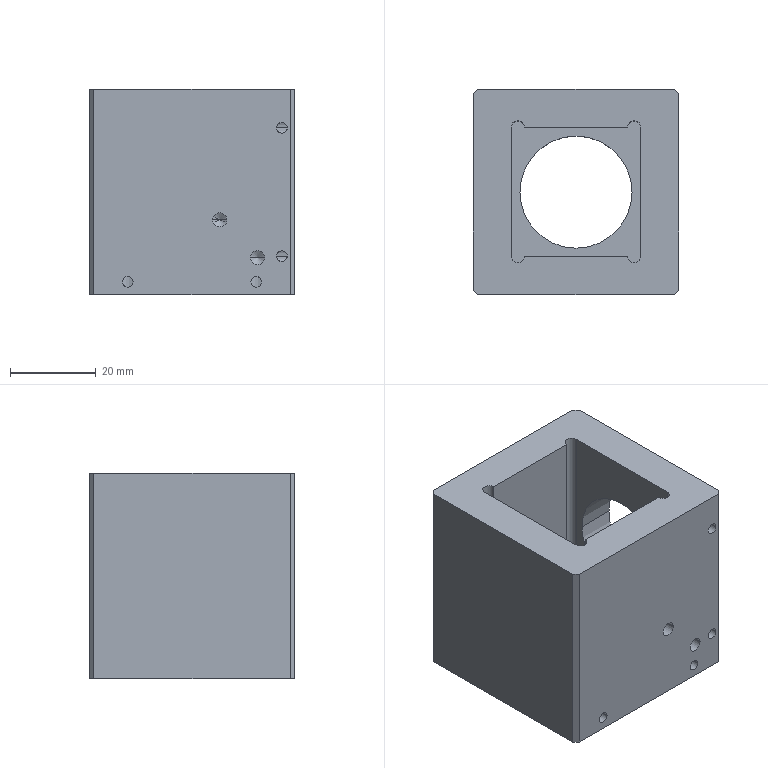NC program | NX | posted with a generic post | part box 48 x 48 x 48 mm
Whole program:
N10 G17 G21 G94 G90
(FLOOR_WALL_COPY_COPY , TOOL : D80)
N12 T19 M6
N14 G54
N16 G17 G0 G90 X-69. Y0. B0. C0. S6500 M3
N18 G43 Z30. H19
N20 Z9.
N22 G94 G1 Z6. F1500.
N24 X-64.
N26 X64.
N28 X69.
N30 Z9.
N32 G0 Z30.
N34 X-69.
N36 Z8.
N38 G1 Z5.
N40 X-64.
N42 X64.
N44 X69.
N46 Z8.
N48 G0 Z30.
N50 X-69.
N52 Z7.
N54 G1 Z4.
N56 X-64.
N58 X64.
N60 X69.
N62 Z7.
N64 G0 Z30.
N66 X-69.
N68 Z6.
N70 G1 Z3.
N72 X-64.
N74 X64.
N76 X69.
N78 Z6.
N80 G0 Z30.
N82 X-69.
N84 Z5.
N86 G1 Z2.
N88 X-64.
N90 X64.
N92 X69.
N94 Z5.
N96 G0 Z30.
N98 X-69.
N100 Z4.
N102 G1 Z1.
N104 X-64.
N106 X64.
N108 X69.
N110 Z4.
N112 G0 Z30.
N114 X-69.
N116 Z3.
N118 G1 Z0.
N120 X-64.
N122 X64.
N124 X69.
N126 Z3.
N128 G0 Z30.
N130 M5
(HOLE_MILLING , TOOL : D10)
N132 T15 M6
N134 G54
N136 G17 G0 G90 X0. Y0. B0. C0. S9500 M3
N138 G43 Z30. H15
N140 Z0.5
N142 G94 G3 X-2. Y2. R2. F2220.
N144 X-4. Y0. R2.
N146 X-4. Y0. Z-0.5 I4. J0.
N148 X-4. Y0. Z-1.5 I4. J0.
N150 X-4. Y0. Z-2.5 I4. J0.
N152 X-4. Y0. Z-3.5 I4. J0.
N154 X-4. Y0. Z-4.5 I4. J0.
N156 X-4. Y0. Z-5.5 I4. J0.
N158 X-4. Y0. Z-6.5 I4. J0.
N160 X-4. Y0. Z-7.5 I4. J0.
N162 X-4. Y0. Z-8.5 I4. J0.
N164 X4. Y0. Z-9. I4. J0.
N166 X0. Y4. R4.
N168 X4. Y0. R-4.
N170 X2. Y2. R2.
N172 X0. Y0. R2.
N174 G0 Z0.5
N176 G3 X-4. Y4. R4.
N178 X-8. Y0. R4.
N180 X-8. Y0. Z-0.5 I8. J0.
N182 X-8. Y0. Z-1.5 I8. J0.
N184 X-8. Y0. Z-2.5 I8. J0.
N186 X-8. Y0. Z-3.5 I8. J0.
N188 X-8. Y0. Z-4.5 I8. J0.
N190 X-8. Y0. Z-5.5 I8. J0.
N192 X-8. Y0. Z-6.5 I8. J0.
N194 X-8. Y0. Z-7.5 I8. J0.
N196 X-8. Y0. Z-8.5 I8. J0.
N198 X8. Y0. Z-9. I8. J0.
N200 X0. Y8. R8.
N202 X8. Y0. R-8.
N204 X4. Y4. R4.
N206 X0. Y0. R4.
N208 G0 Z30.
N210 M5
(ZLEVEL_PROFILE_COPY_1_COPY_COPY_1_COPY_COPY_COPY , TOOL : D10JING)
N212 T14 M6
N214 G54
N216 G17 G0 G90 X-1.153 Y5.648 B0. C0. S9500 M3
N218 G43 Z30. H14
N220 Z-8.
N222 G94 G1 Z-9. F1000.
N224 X-4.229 Y6.473
N226 G3 X-5.195 Y6.214 R1.
N228 G1 X-6.212 Y5.198 F1200.
N230 G3 X-7.759 Y-2.325 R8.1
N232 G1 X-7.732 Y-2.339
N234 X-7.743 Y-2.379
N236 G3 X-6.214 Y-5.195 R8.1
N238 G1 X-5.198 Y-6.212
N240 G3 X5.195 Y-6.214 R8.1
N242 G1 X6.212 Y-5.198
N244 G3 X7.759 Y2.325 R8.1
N246 G1 X7.732 Y2.339
N248 X7.743 Y2.379
N250 G3 X6.214 Y5.195 R8.1
N252 G1 X5.198 Y6.212
N254 G3 X-2.325 Y7.759 R8.1
N256 G1 X-2.339 Y7.732
N258 X-2.379 Y7.743
N260 G3 X-5.195 Y6.214 R8.1
N262 X-5.539 Y5.275 R1.
N264 G1 X-5.181 Y3.221
N266 Z-8.
N268 G0 Z30.
N270 M5
(HOLE_MILLING_1 , TOOL : D4)
N272 T11 M6
N274 G54
N276 G17 G0 G90 X-15. Y15. B0. C0. S9500 M3
N278 G43 Z30. H11
N280 Z0.5
N282 G94 G3 X-15.45 Y15.45 R0.45 F1650.
N284 X-15.9 Y15. R0.45
N286 X-15.9 Y15. Z0.1 I0.9 J0.
N288 X-15.9 Y15. Z-0.3 I0.9 J0.
N290 X-15.9 Y15. Z-0.7 I0.9 J0.
N292 X-15.9 Y15. Z-1.1 I0.9 J0.
N294 X-15.9 Y15. Z-1.5 I0.9 J0.
N296 X-15.9 Y15. Z-1.9 I0.9 J0.
N298 X-15.9 Y15. Z-2.3 I0.9 J0.
N300 X-15.9 Y15. Z-2.7 I0.9 J0.
N302 X-15.9 Y15. Z-3.1 I0.9 J0.
N304 X-15.9 Y15. Z-3.5 I0.9 J0.
N306 X-15.9 Y15. Z-3.9 I0.9 J0.
N308 X-15.9 Y15. Z-4.3 I0.9 J0.
N310 X-15.9 Y15. Z-4.7 I0.9 J0.
N312 X-15.9 Y15. Z-5.1 I0.9 J0.
N314 X-15.9 Y15. Z-5.5 I0.9 J0.
N316 X-15. Y14.1 R0.9
N318 X-15.9 Y15. R-0.9
N320 X-15.45 Y14.55 R0.45
N322 X-15. Y15. R0.45
N324 G0 Z30.
N326 Y-15.
N328 Z0.5
N330 G3 X-15.45 Y-14.55 R0.45
N332 X-15.9 Y-15. R0.45
N334 X-15.9 Y-15. Z0.1 I0.9 J0.
N336 X-15.9 Y-15. Z-0.3 I0.9 J0.
N338 X-15.9 Y-15. Z-0.7 I0.9 J0.
N340 X-15.9 Y-15. Z-1.1 I0.9 J0.
N342 X-15.9 Y-15. Z-1.5 I0.9 J0.
N344 X-15.9 Y-15. Z-1.9 I0.9 J0.
N346 X-15.9 Y-15. Z-2.3 I0.9 J0.
N348 X-15.9 Y-15. Z-2.7 I0.9 J0.
N350 X-15.9 Y-15. Z-3.1 I0.9 J0.
N352 X-15.9 Y-15. Z-3.5 I0.9 J0.
N354 X-15.9 Y-15. Z-3.9 I0.9 J0.
N356 X-15.9 Y-15. Z-4.3 I0.9 J0.
N358 X-15.9 Y-15. Z-4.7 I0.9 J0.
N360 X-15.9 Y-15. Z-5.1 I0.9 J0.
N362 X-15.9 Y-15. Z-5.5 I0.9 J0.
N364 X-15. Y-15.9 R0.9
N366 X-15.9 Y-15. R-0.9
N368 X-15.45 Y-15.45 R0.45
N370 X-15. Y-15. R0.45
N372 G0 Z30.
N374 X15.
N376 Z0.5
N378 G3 X14.55 Y-14.55 R0.45
N380 X14.1 Y-15. R0.45
N382 X14.1 Y-15. Z0.1 I0.9 J0.
N384 X14.1 Y-15. Z-0.3 I0.9 J0.
N386 X14.1 Y-15. Z-0.7 I0.9 J0.
N388 X14.1 Y-15. Z-1.1 I0.9 J0.
N390 X14.1 Y-15. Z-1.5 I0.9 J0.
N392 X14.1 Y-15. Z-1.9 I0.9 J0.
N394 X14.1 Y-15. Z-2.3 I0.9 J0.
N396 X14.1 Y-15. Z-2.7 I0.9 J0.
N398 X14.1 Y-15. Z-3.1 I0.9 J0.
N400 X14.1 Y-15. Z-3.5 I0.9 J0.
N402 X14.1 Y-15. Z-3.9 I0.9 J0.
N404 X14.1 Y-15. Z-4.3 I0.9 J0.
N406 X14.1 Y-15. Z-4.7 I0.9 J0.
N408 X14.1 Y-15. Z-5.1 I0.9 J0.
N410 X14.1 Y-15. Z-5.5 I0.9 J0.
N412 X15. Y-15.9 R0.9
N414 X14.1 Y-15. R-0.9
N416 X14.55 Y-15.45 R0.45
N418 X15. Y-15. R0.45
N420 G0 Z30.
N422 Y15.
N424 Z0.5
N426 G3 X14.55 Y15.45 R0.45
N428 X14.1 Y15. R0.45
N430 X14.1 Y15. Z0.1 I0.9 J0.
N432 X14.1 Y15. Z-0.3 I0.9 J0.
N434 X14.1 Y15. Z-0.7 I0.9 J0.
N436 X14.1 Y15. Z-1.1 I0.9 J0.
N438 X14.1 Y15. Z-1.5 I0.9 J0.
N440 X14.1 Y15. Z-1.9 I0.9 J0.
N442 X14.1 Y15. Z-2.3 I0.9 J0.
N444 X14.1 Y15. Z-2.7 I0.9 J0.
N446 X14.1 Y15. Z-3.1 I0.9 J0.
N448 X14.1 Y15. Z-3.5 I0.9 J0.
N450 X14.1 Y15. Z-3.9 I0.9 J0.
N452 X14.1 Y15. Z-4.3 I0.9 J0.
N454 X14.1 Y15. Z-4.7 I0.9 J0.
N456 X14.1 Y15. Z-5.1 I0.9 J0.
N458 X14.1 Y15. Z-5.5 I0.9 J0.
N460 X15. Y14.1 R0.9
N462 X14.1 Y15. R-0.9
N464 X14.55 Y14.55 R0.45
N466 X15. Y15. R0.45
N468 G0 Z30.
N470 M5
(PLANAR_MILL_COPY_COPY_COPY_COPY_COPY_COPY_1_COPY_1_COPY , TOOL : D6A45)
N472 T01 M6
N474 G54
N476 G17 G0 G90 X15.866 Y16.7 B0. C0. S9500 M3
N478 G43 Z30. H1
N480 Z0.5
N482 G94 G1 Z-1. F1250.
N484 G3 X15. Y17.2 R1.
N486 X12.8 Y15. R2.2
N488 X15. Y17.2 R-2.2
N490 X14.134 Y16.7 R1.
N492 G1 Z0.5
N494 G0 Z30.
N496 X-0.866 Y25.3
N498 Z0.5
N500 G1 Z-1.
N502 G3 X0. Y24.8 R1.
N504 G1 X23.
N506 G2 X23.566 Y24.566 R0.8
N508 G1 X24.566 Y23.566
N510 G2 X24.8 Y23. R0.8
N512 G1 Y-23.
N514 G2 X24.566 Y-23.566 R0.8
N516 G1 X23.566 Y-24.566
N518 G2 X23. Y-24.8 R0.8
N520 G1 X-23.
N522 G2 X-23.566 Y-24.566 R0.8
N524 G1 X-24.566 Y-23.566
N526 G2 X-24.8 Y-23. R0.8
N528 G1 Y23.
N530 G2 X-24.566 Y23.566 R0.8
N532 G1 X-23.566 Y24.566
N534 G2 X-23. Y24.8 R0.8
N536 G1 X0.
N538 G3 X0.866 Y25.3 R1.
N540 G1 Z0.5
N542 G0 Z30.
N544 X-14.134 Y16.7
N546 Z0.5
N548 G1 Z-1.
N550 G3 X-15. Y17.2 R1.
N552 X-17.2 Y15. R2.2
N554 X-15. Y17.2 R-2.2
N556 X-15.866 Y16.7 R1.
N558 G1 Z0.5
N560 G0 Z30.
N562 X0.866 Y11.8
N564 Z0.5
N566 G1 Z-1.
N568 G3 X0. Y12.3 R1.
N570 X-12.3 Y0. R12.3
N572 X0. Y12.3 R-12.3
N574 X-0.866 Y11.8 R1.
N576 G1 Z0.5
N578 G0 Z30.
N580 X-16.7 Y-14.134
N582 Z0.5
N584 G1 Z-1.
N586 G3 X-17.2 Y-15. R1.
N588 X-15. Y-17.2 R2.2
N590 X-17.2 Y-15. R-2.2
N592 X-16.7 Y-15.866 R1.
N594 G1 Z0.5
N596 G0 Z30.
N598 X14.134 Y-16.7
N600 Z0.5
N602 G1 Z-1.
N604 G3 X15. Y-17.2 R1.
N606 X17.2 Y-15. R2.2
N608 X15. Y-17.2 R-2.2
N610 X15.866 Y-16.7 R1.
N612 G1 Z0.5
N614 G0 Z30.
N616 M5
(刀补11 , TOOL : D4)
N618 T11 M6
N620 G54
N622 G17 G0 G90 X-15. Y15. B0. C0. S9500 M3
N624 G43 Z30. H11
N626 Z0.5
N628 G41 G94 G1 X-15.004 Y15.1 F1000. D11
N630 G3 X-15.95 Y15. R0.478
N632 X-15.95 Y15. Z-1.5 I0.95 J0.
N634 X-15.95 Y15. Z-3.5 I0.95 J0.
N636 X-15.95 Y15. Z-5.5 I0.95 J0.
N638 X-15. Y14.05 R0.95
N640 X-15.95 Y15. R-0.95
N642 X-15.004 Y14.9 R0.478
N644 G40
N646 G1 X-15. Y15.
N648 G0 Z30.
N650 Y-15.
N652 Z0.5
N654 G41 G1 X-15.004 Y-14.9
N656 G3 X-15.95 Y-15. R0.478
N658 X-15.95 Y-15. Z-1.5 I0.95 J0.
N660 X-15.95 Y-15. Z-3.5 I0.95 J0.
N662 X-15.95 Y-15. Z-5.5 I0.95 J0.
N664 X-15. Y-15.95 R0.95
N666 X-15.95 Y-15. R-0.95
N668 X-15.004 Y-15.1 R0.478
N670 G40
N672 G1 X-15. Y-15.
N674 G0 Z30.
N676 X15.
N678 Z0.5
N680 G41 G1 X14.996 Y-14.9
N682 G3 X14.05 Y-15. R0.478
N684 X14.05 Y-15. Z-1.5 I0.95 J0.
N686 X14.05 Y-15. Z-3.5 I0.95 J0.
N688 X14.05 Y-15. Z-5.5 I0.95 J0.
N690 X15. Y-15.95 R0.95
N692 X14.05 Y-15. R-0.95
N694 X14.996 Y-15.1 R0.478
N696 G40
N698 G1 X15. Y-15.
N700 G0 Z30.
N702 Y15.
N704 Z0.5
N706 G41 G1 X14.996 Y15.1
N708 G3 X14.05 Y15. R0.478
N710 X14.05 Y15. Z-1.5 I0.95 J0.
N712 X14.05 Y15. Z-3.5 I0.95 J0.
N714 X14.05 Y15. Z-5.5 I0.95 J0.
N716 X15. Y14.05 R0.95
N718 X14.05 Y15. R-0.95
N720 X14.996 Y14.9 R0.478
N722 G40
N724 G1 X15. Y15.
N726 G0 Z30.
N728 M5
N730 M2